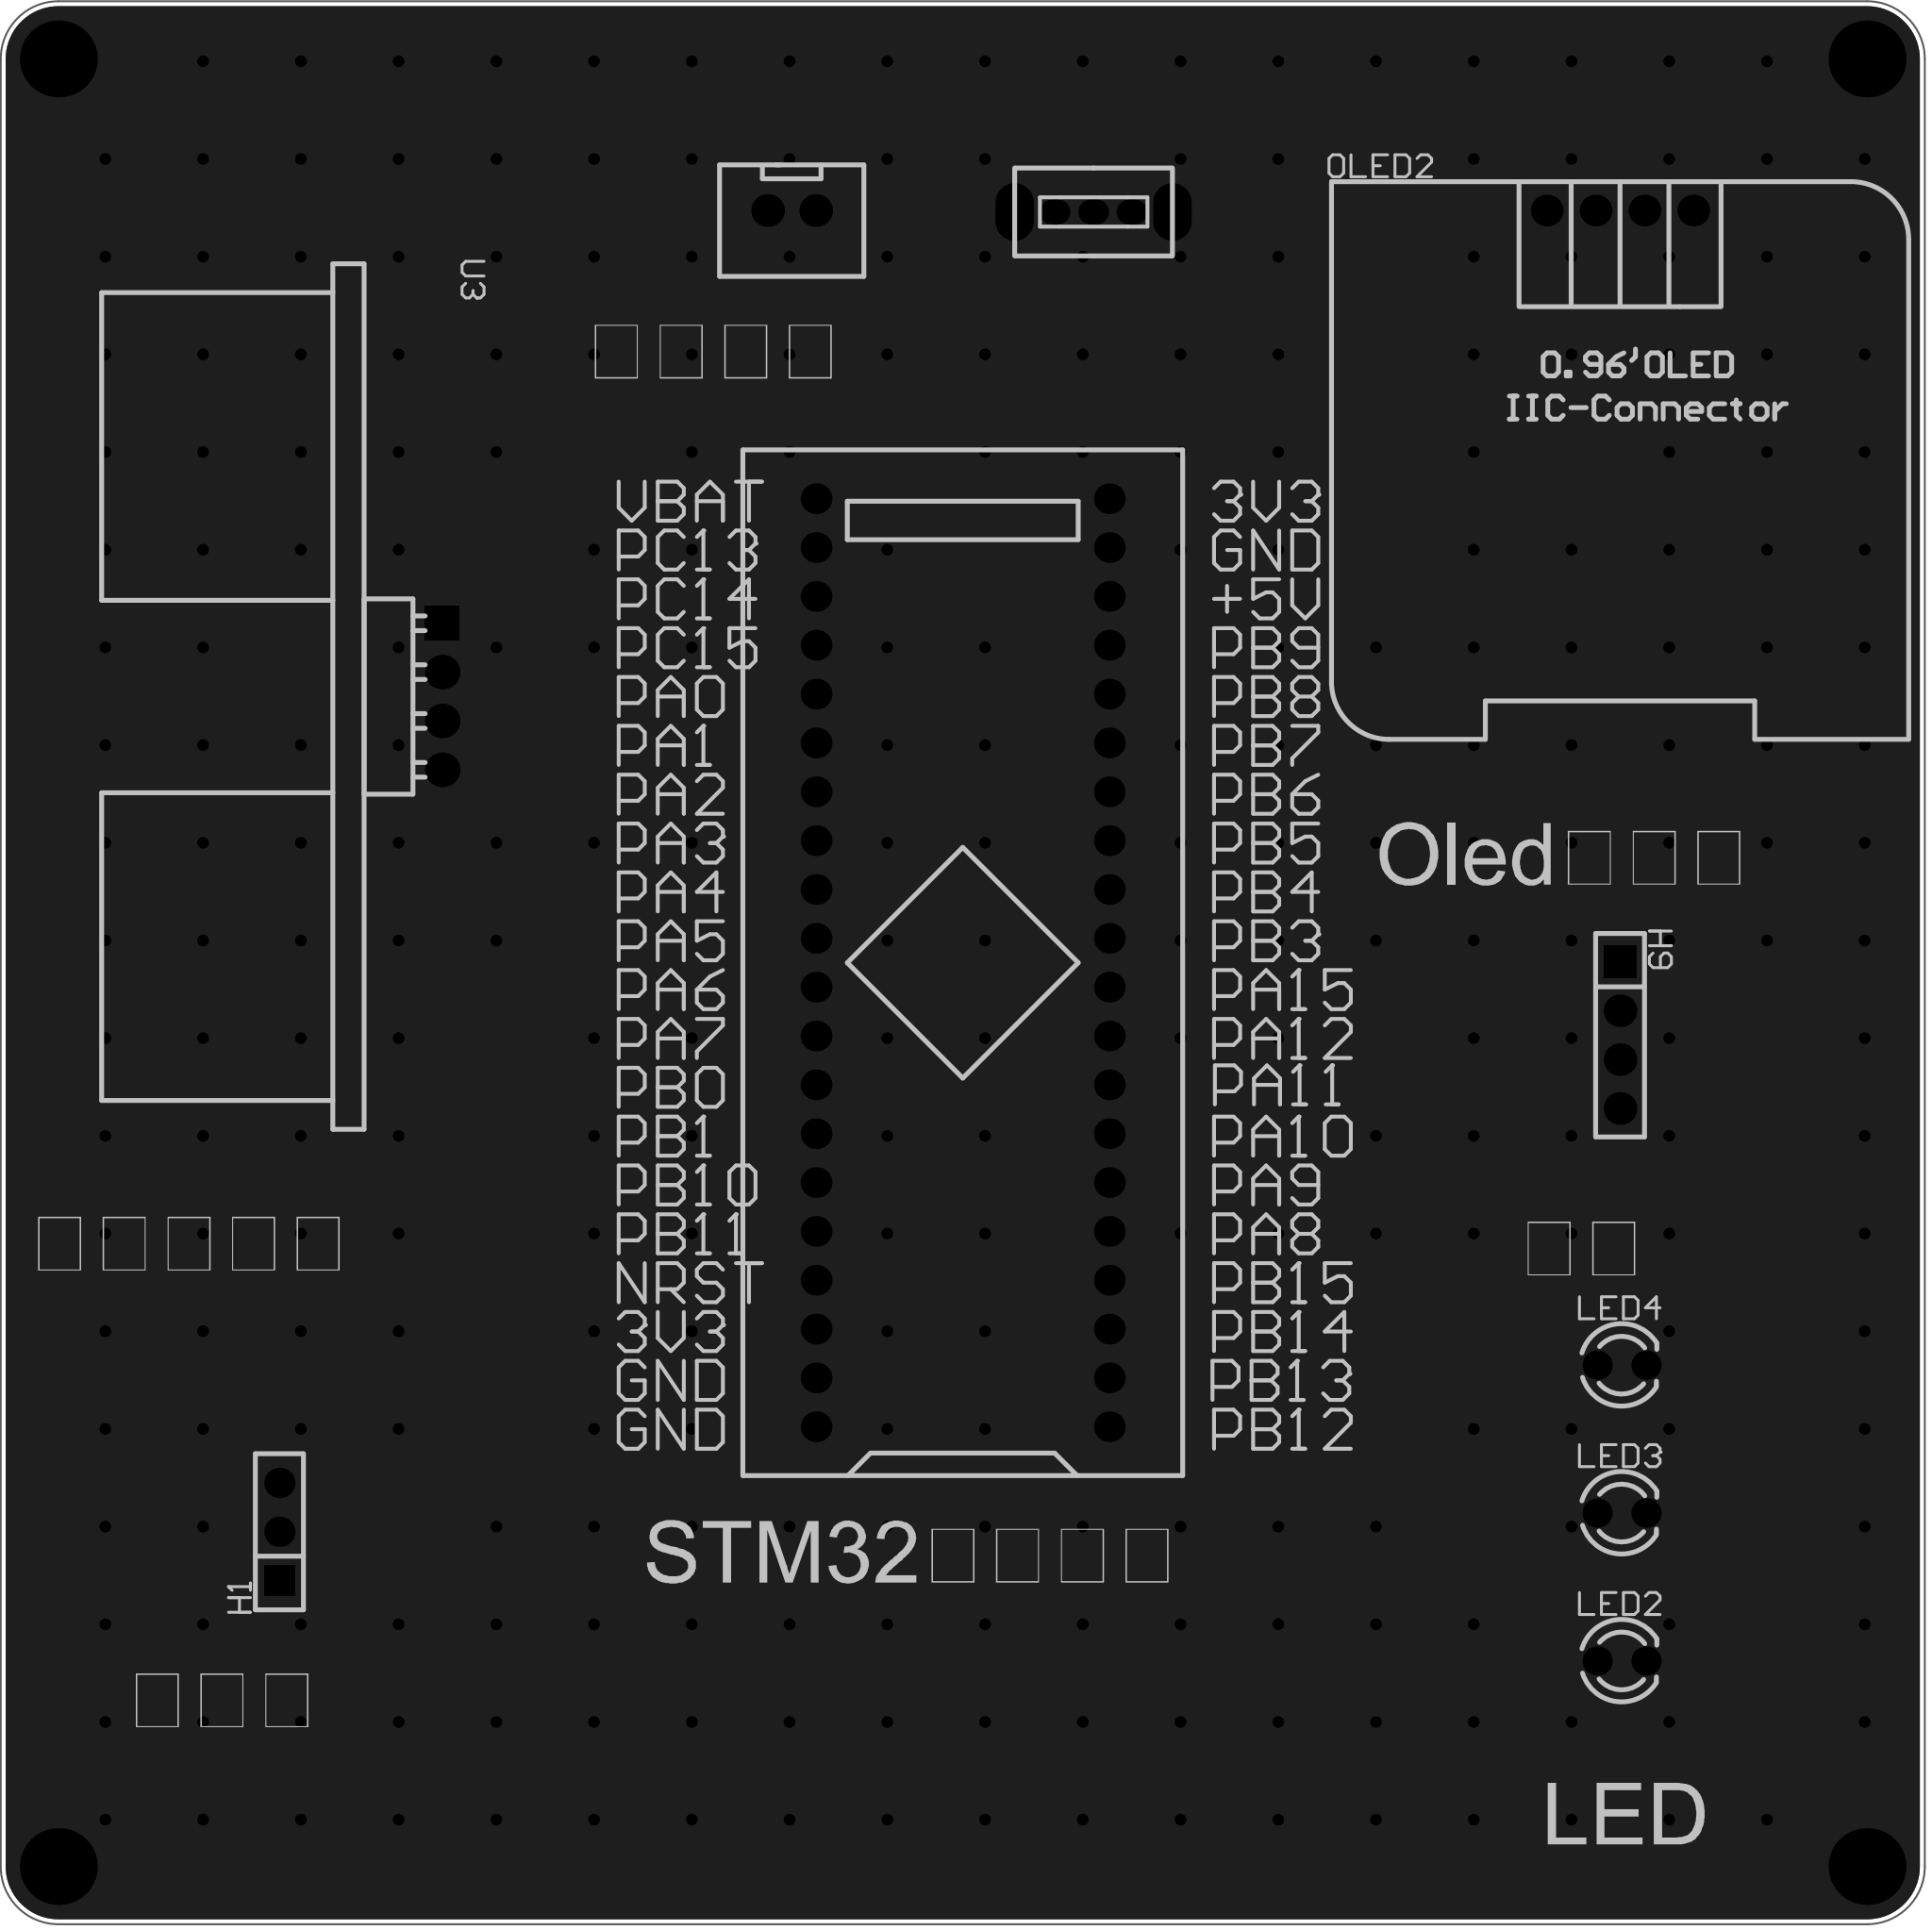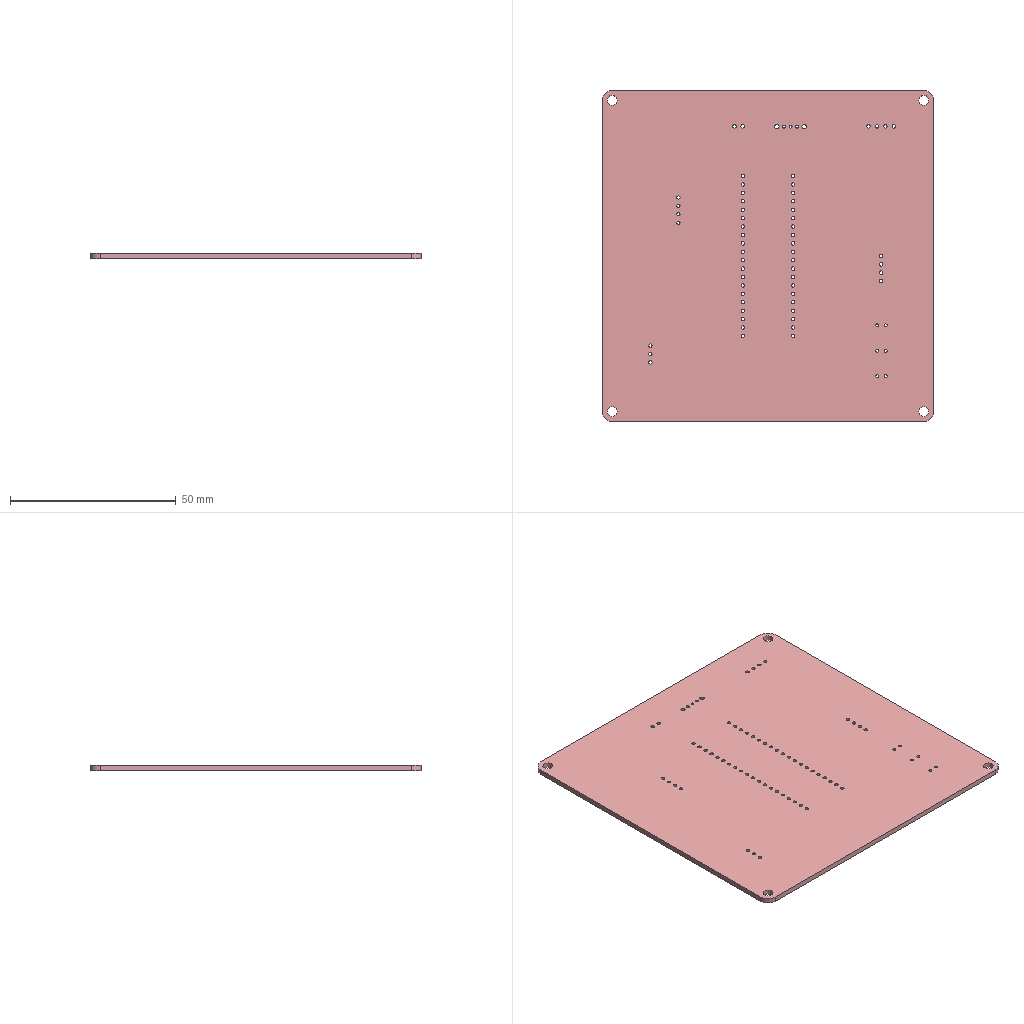Circuit board layout | Altium Designer | box 100 x 100 x 1.6 mm
Layer stack:
# Altium Designer layer stack of  (unit mm; dielectric type: 0 none, 1 core, 2 prepreg, 3 surface material)
index,name,kind,layer,copper_thickness_mm,dielectric_type,dielectric_thickness_mm,dielectric_material,dielectric_constant
0,Top Paste Mask Layer,other,,,,,,
1,Top Silkscreen Layer,other,,,,,,
2,Top Solder Mask Layer,dielectric,,,3,0.01,,3.3
3,Top Layer,copper,Top Layer,0.035,,,,
4,Dielectric1,dielectric,,,3,1.51,FR4,4.5
5,Bottom Layer,copper,Bottom Layer,0.035,,,,
6,Bottom Solder Mask Layer,dielectric,,,3,0.01,,3.3
7,Bottom Silkscreen Layer,other,,,,,,
8,Bottom Paste Mask Layer,other,,,,,,
# drill layer pairs: low layer,high layer
drill_pair,Top Layer,Bottom Layer
Part placement:
Designator,Comment,Layer,Footprint,Center-X(mm),Center-Y(mm),Rotation
U1,STM32F103C8T6-Card,TopLayer,CONN-TH_L53.3-W22.9_STM32F103C8T6-CARD,141.351,130.937,90
CN4,XH2.54*2P_直插,TopLayer,CONN-TH_2P-P2.50-XH2.54-2P,132.461,170.053,0
SW5,,TopLayer,拨动开关,148.148,169.978,180
OLED2,,TopLayer,0.96OLED_4P,175.514,170.053,0
H1,,TopLayer,HDR-TH_3P-P2.54-V-F,105.835,101.346,90
H9,,TopLayer,HDR-TH_4P-P2.54-V-F,175.514,127.168,270
LED2,,TopLayer,LED_TH-3mm,175.593,94.63,0
LED3,,TopLayer,LED_TH-3mm,175.593,102.32,0
LED4,,TopLayer,LED_TH-3mm,175.593,110.01,0
U3,HC-SR04,TopLayer,TH_HC-SR04V,114.3,144.78,270
Pad and via stacks:
# Altium Designer via and pad stacks of  (unit mm). Each distinct definition once, with the count of objects using it.
# via: kind,start_layer,end_layer,hole_mm,diameter_mm,mode(0 simple;1 top-mid-bottom;2 full stack),diameter_per_layer,count,example_net
# pad: kind,layer,hole_mm,hole_type(0 round;1 square;2 slot),plating,top_size,top_shape(1 round;2 rect;3 octagon;9 rounded rect),mid_size,bottom_size,mode,footprint,size_per_layer,count,example
pad,Multi-Layer,3,0,plated,4x4,1,4x4,4x4,0,,,4,1
pad,Multi-Layer,1,0,plated,1.6x1.6,1,1.6x1.6,1.6x1.6,0,CONN-TH_L53.3-W22.9_STM32F103C8T6-CARD,,40,U1.1
pad,Multi-Layer,1.05,0,plated,1.7x1.7,1,1.7x1.7,1.7x1.7,0,CONN-TH_2P-P2.50-XH2.54-2P,,2,CN4.2
pad,Multi-Layer,0.8992,0,plated,1.6x1.3,1,1.6x1.3,1.6x1.3,0,\u00B2\u00A6\u00B6\u00AF\u00BF\u00AA\u00B9\u00D8,,3,SW5.1
pad,Multi-Layer,1.3,0,plated,3x1.999,1,3x1.999,3x1.999,0,\u00B2\u00A6\u00B6\u00AF\u00BF\u00AA\u00B9\u00D8,,2,SW5.4
pad,Multi-Layer,1,0,plated,1.65x1.65,1,1.65x1.65,1.65x1.65,0,0.96OLED_4P,,4,OLED2.4
pad,Multi-Layer,1.02,0,plated,1.575x1.575,1,1.575x1.575,1.575x1.575,0,HDR-TH_3P-P2.54-V-F,,2,H1.3
pad,Multi-Layer,1.02,0,plated,1.575x1.575,2,1.575x1.575,1.575x1.575,0,HDR-TH_3P-P2.54-V-F,,1,H1.1
pad,Multi-Layer,1.1,0,plated,1.7x1.7,2,1.7x1.7,1.7x1.7,0,HDR-TH_4P-P2.54-V-F,,1,H9.1
pad,Multi-Layer,1.1,0,plated,1.7x1.7,1,1.7x1.7,1.7x1.7,0,HDR-TH_4P-P2.54-V-F,,3,H9.2
pad,Multi-Layer,0.9144,0,plated,1.524x1.524,1,1.524x1.524,1.524x1.524,0,LED_TH-3mm,,6,LED2.1
pad,Multi-Layer,1.001,0,plated,1.8x1.8,1,1.8x1.8,1.8x1.8,0,TH_HC-SR04V,,3,U3.4
pad,Multi-Layer,1.001,0,plated,1.8x1.8,2,1.8x1.8,1.8x1.8,0,TH_HC-SR04V,,1,U3.1
via,Top Layer,Bottom Layer,0.3048,0.61,0,,291,GND
Copper pours:
name,layer,net,type(0 solid;1 hatched;2 none)
Bottom Layer-GND,Bottom Layer,GND,0
Top Layer-GND,Top Layer,GND,0
Design rules, without the lines most boards share:
# Altium Designer design rules of  (exported by Altium Designer, unit mm)
# columns: name | kind | enabled | priority | scope1 | scope2 | descriptor | typed fields (field=value)
Copper_copperRegion_copperThickness1oz | 0 | disabled | 4 | All | All | Clearance Constraint (Gap=5.984mil) (Disabled)(All),(All) | gap=0.152
Copper_copperRegion_copperThickness1oz_1 | 63 | disabled | 4 | All | All | Board Clearance Constraint (Gap=0mil) (Disabled)(All) |
Copper_copperRegion_Copper_copperRegion | 0 | disabled | 5 | All | All | Clearance Constraint (Gap=5.984mil) (Disabled)(All),(All) | gap=0.152
Copper_copperRegion_Copper_copperRegion_1 | 63 | disabled | 5 | All | All | Board Clearance Constraint (Gap=0mil) (Disabled)(All) |
copperThickness1oz | 0 | enabled | 6 | All | All | Clearance Constraint (Gap=5.984mil) (All),(All) | gap=0.152
copperThickness1oz_1 | 63 | enabled | 6 | All | All | Board Clearance Constraint (Gap=0mil) (All) |
copperRegion_copperThickness1oz | 20 | disabled | 1 | All | All | Polygon Connect Rule(Relief Connect )(Conductor Width=10mil) (Relief Angle=90 Angle) (Entries=4) (Air Gap Width=10mil) (Disabled)(All),(All) | connect_style(0=relief,1=direct,2=none)=0 relief_conductor_width=0.254 relief_entries=4
copperRegion_Copper_copperRegion | 20 | disabled | 2 | All | All | Polygon Connect Rule(Relief Connect )(Conductor Width=10mil) (Relief Angle=90 Angle) (Entries=4) (Air Gap Width=10mil) (Disabled)(All),(All) | connect_style(0=relief,1=direct,2=none)=0 relief_conductor_width=0.254 relief_entries=4
copperRegion | 20 | enabled | 3 | All | All | Polygon Connect Rule(Relief Connect )(Conductor Width=10mil) (Relief Angle=90 Angle) (Entries=4) (Air Gap Width=10mil) (All),(All) | connect_style(0=relief,1=direct,2=none)=0 relief_conductor_width=0.254 relief_entries=4